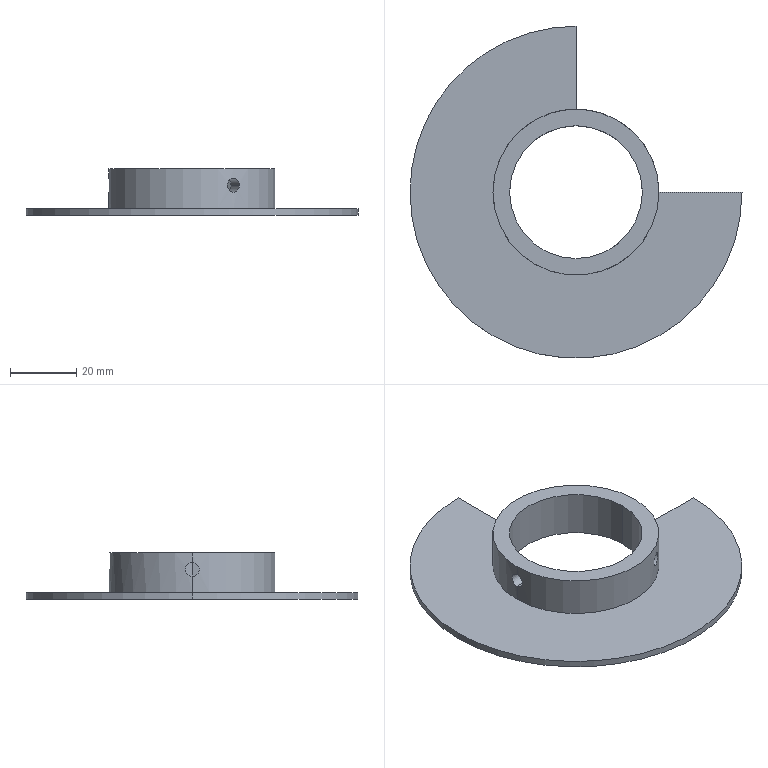Part | STEP file | BB013A02M-04-39A | 1 solid | 15 faces | box 100 x 100 x 14 mm | volume 18593 mm3 | cylinder 10 | plane 5 | commonest cylinder face diameters 4.2 x4 40 x2 50 x2 100 x2